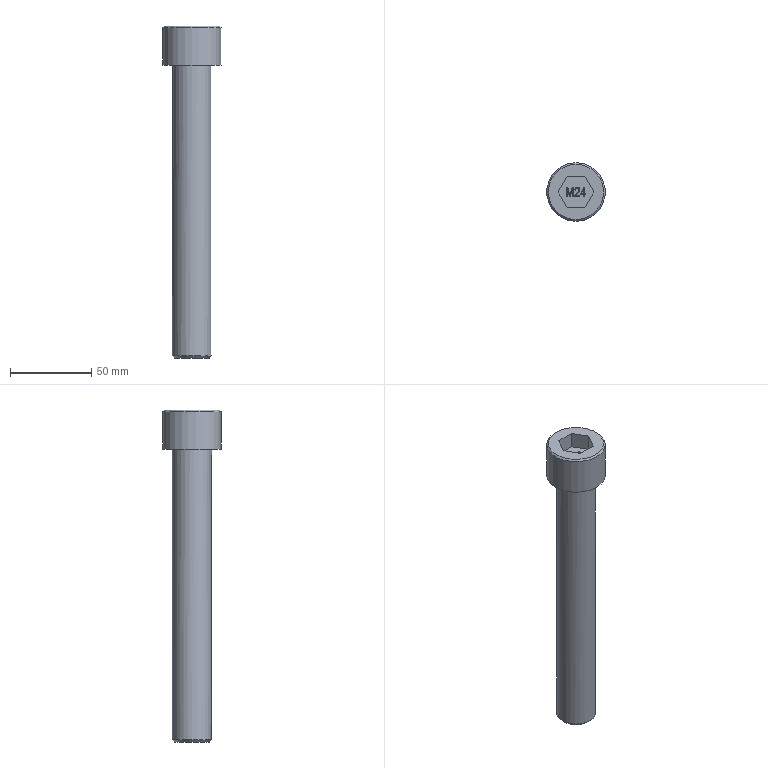Part | STEP file | M24-2 | 1 solid | 51 faces | box 36 x 36 x 204 mm | volume 102621 mm3 | plane 43 | other 4 | cylinder 2 | cone 2 | commonest cylinder face diameters 24 x1 36 x1